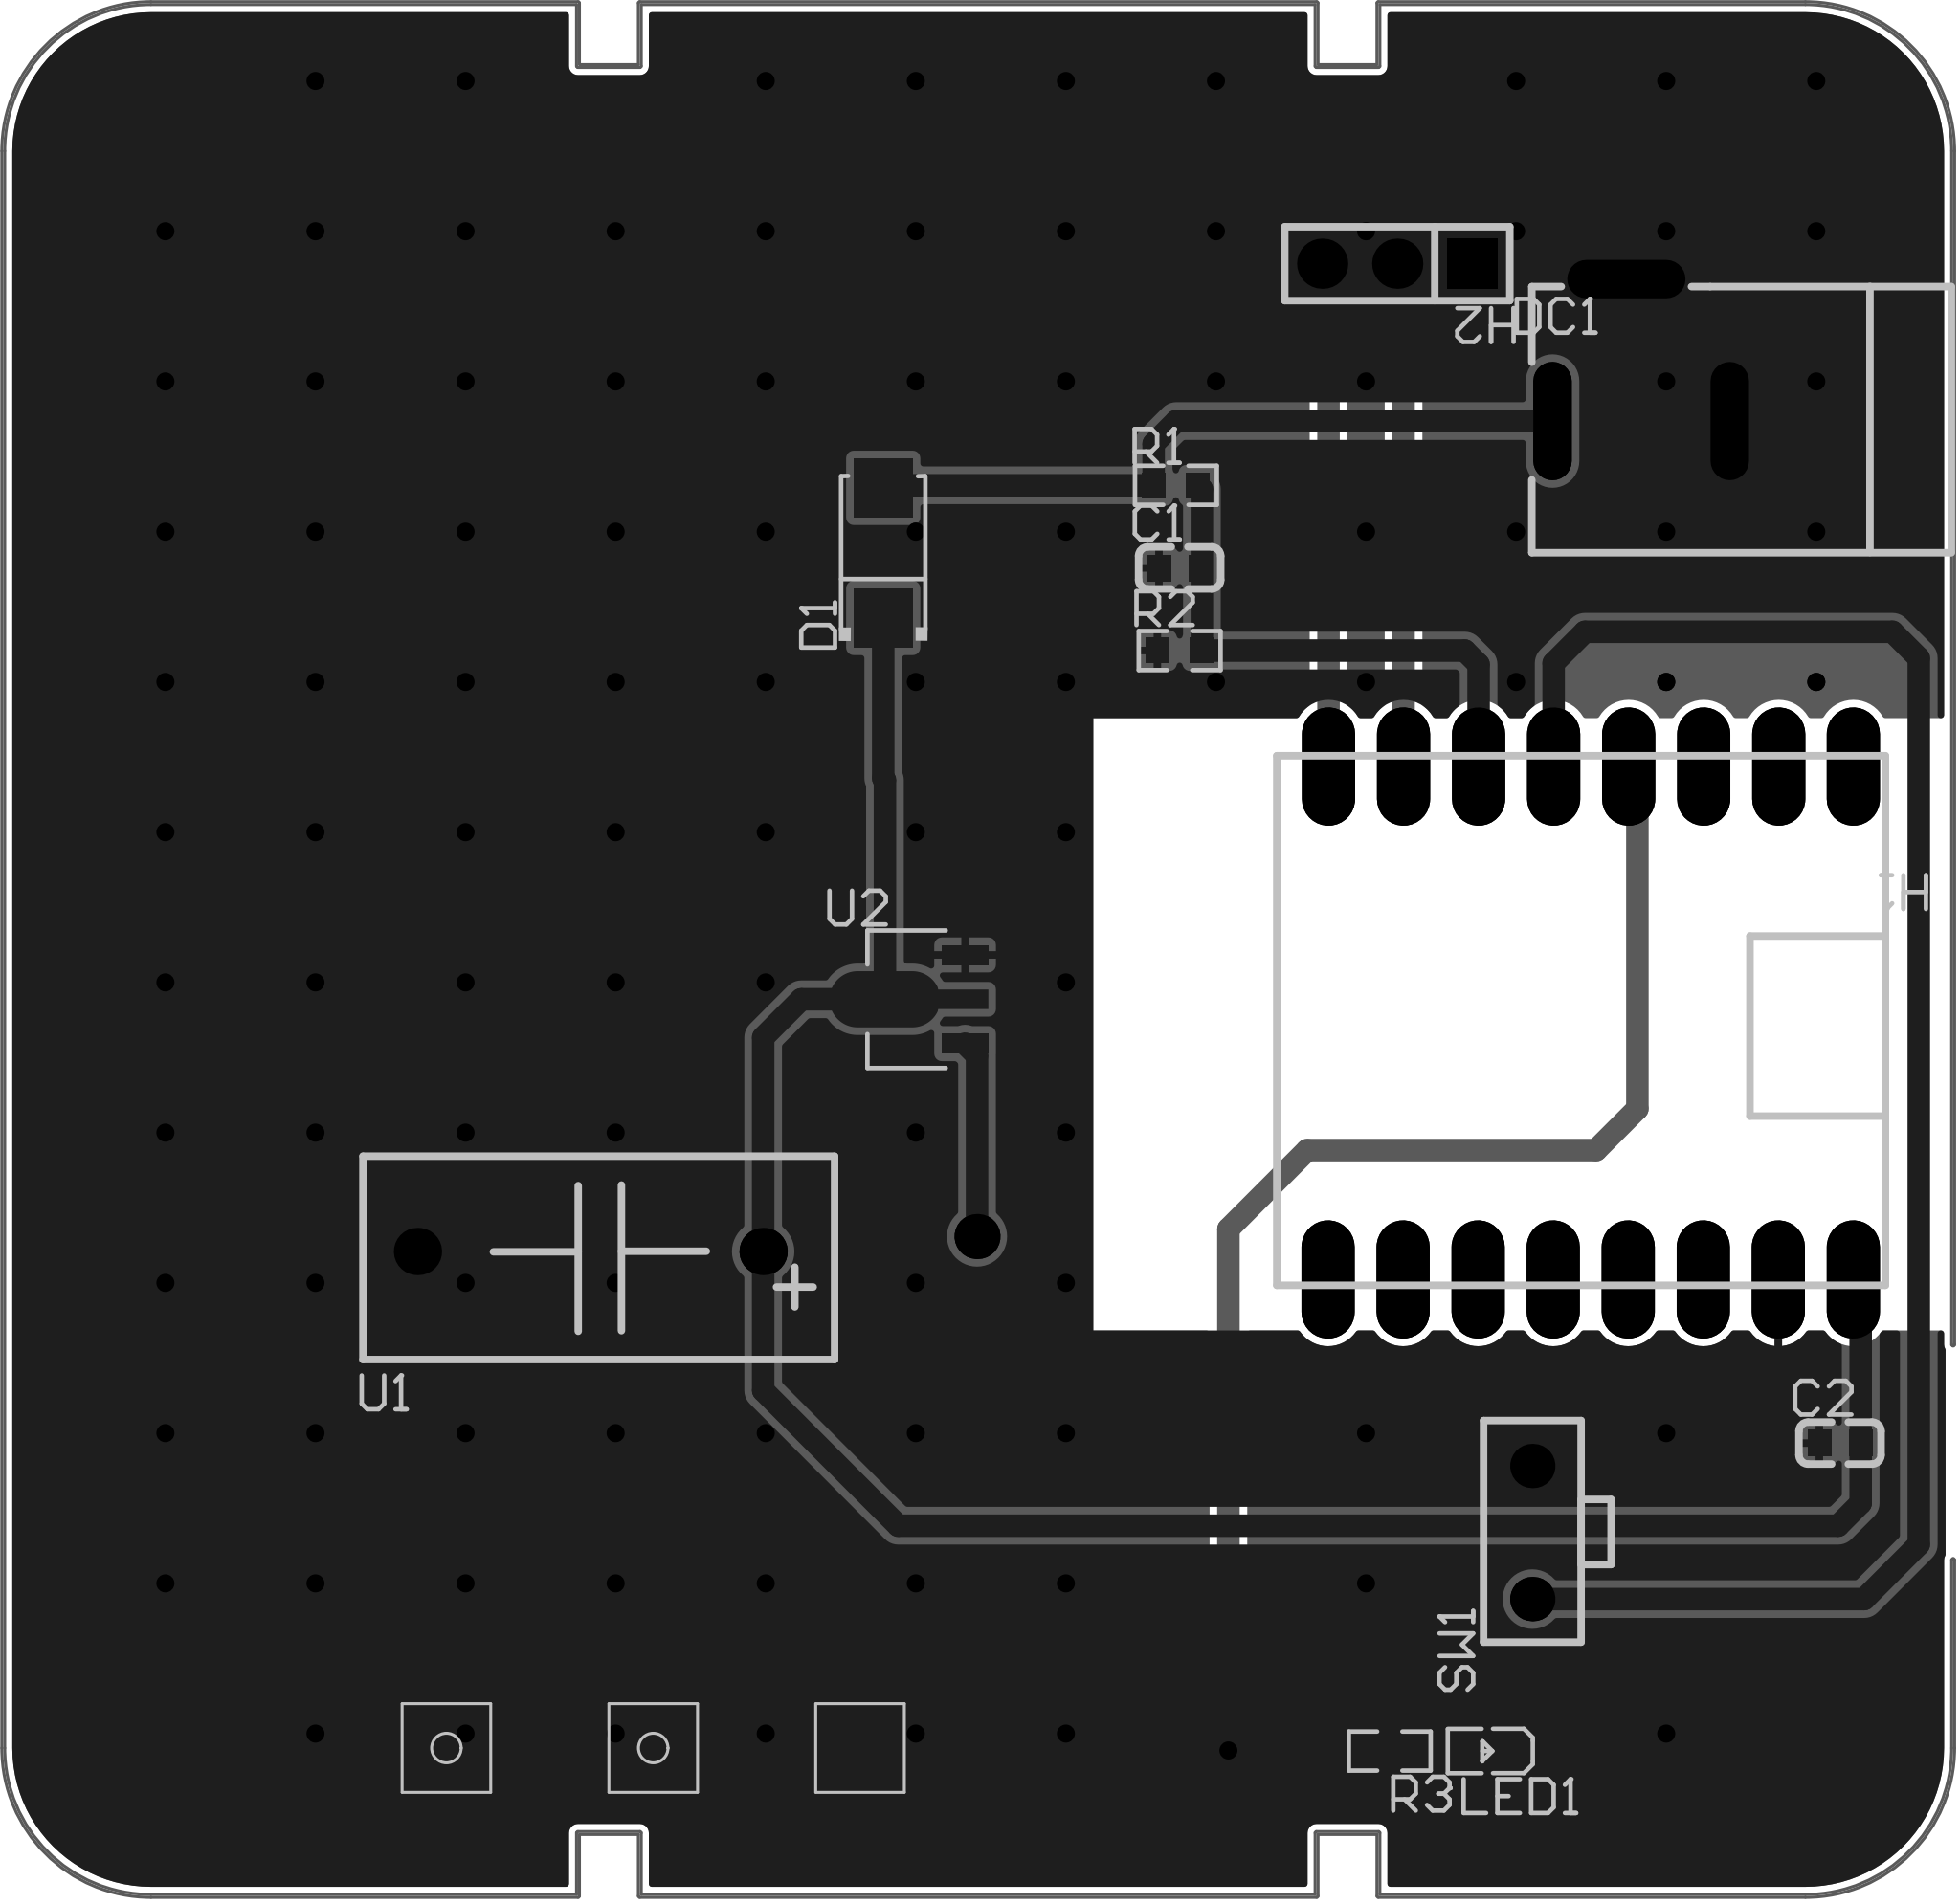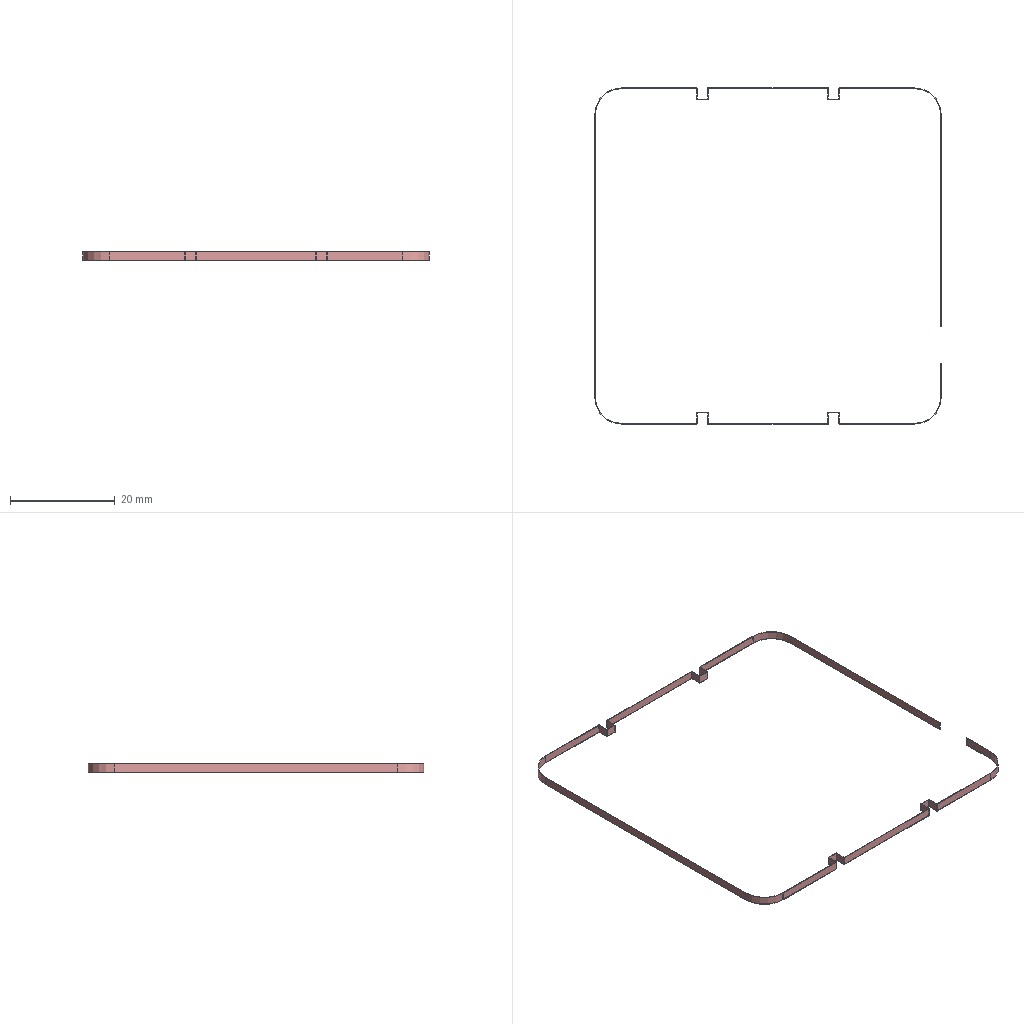Circuit board layout | Altium Designer | box 66.1 x 64.1 x 1.6 mm
Layer stack:
# Altium Designer layer stack of  (unit mm; dielectric type: 0 none, 1 core, 2 prepreg, 3 surface material)
index,name,kind,layer,copper_thickness_mm,dielectric_type,dielectric_thickness_mm,dielectric_material,dielectric_constant
0,Top Paste Mask Layer,other,,,,,,
1,Top Silkscreen Layer,other,,,,,,
2,Top Solder Mask Layer,dielectric,,,3,0.01,,3.3
3,Top Layer,copper,Top Layer,0.035,,,,
4,Dielectric1,dielectric,,,3,1.51,FR4,4.5
5,Bottom Layer,copper,Bottom Layer,0.035,,,,
6,Bottom Solder Mask Layer,dielectric,,,3,0.01,,3.3
7,Bottom Silkscreen Layer,other,,,,,,
8,Bottom Paste Mask Layer,other,,,,,,
# drill layer pairs: low layer,high layer
drill_pair,Top Layer,Bottom Layer
Part placement:
Designator,Comment,Layer,Footprint,Center-X(mm),Center-Y(mm),Rotation
C1,100nF,TopLayer,C0603,125.984,131.191,0
C2,100nF,TopLayer,C0603,148.336,101.6,0
D1,SS34,TopLayer,SMA_L4.3-W2.6-LS5.2-RD,115.951,131.699,90
H1,,TopLayer,HDR-TH_16P-P2.54-V-F-R2-C8-S2.54-1,139.898,115.803,180
R1,10K,TopLayer,R0603,125.857,133.985,180
R2,15K,TopLayer,R0603,125.984,128.397,0
R3,1K,TopLayer,R0603,133.096,91.186,0
U1,2F,TopLayer,CAP-TH_BD8.0-P3.50-D0.6-FD_GDC02R7R205LD0816,106.037,108.077,180
U2,HT7033A-1,TopLayer,SOT-89-3_L4.5-W2.5-P1.50-LS4.2-BR,117.561,116.606,0
DC1,,TopLayer,DC-2.0,141.605,138.557,0
H2,,TopLayer,HDR-TH_3P-P2.54-V-M,133.35,141.478,180
LED1,,TopLayer,LED_0603,136.449,91.194,180
SW1,,TopLayer,Key_TH_3.5x6x4.3,137.922,98.574,90
Pad and via stacks:
# Altium Designer via and pad stacks of  (unit mm). Each distinct definition once, with the count of objects using it.
# via: kind,start_layer,end_layer,hole_mm,diameter_mm,mode(0 simple;1 top-mid-bottom;2 full stack),diameter_per_layer,count,example_net
# pad: kind,layer,hole_mm,hole_type(0 round;1 square;2 slot),plating,top_size,top_shape(1 round;2 rect;3 octagon;9 rounded rect),mid_size,bottom_size,mode,footprint,size_per_layer,count,example
pad,Top Layer,0,0,plated,0.8x0.9,2,0.8x0.9,0.8x0.9,0,C0603,,4,C1.2
pad,Top Layer,0,0,plated,2x2,2,2x2,2x2,0,SMA_L4.3-W2.6-LS5.2-RD,,2,D1.2
pad,Top Layer,0,0,plated,0.8065x0.864,2,0.8065x0.864,0.8065x0.864,0,R0603,,6,R1.2
pad,Top Layer,0,0,plated,1.575x0.672,2,1.575x0.672,1.575x0.672,0,SOT-89-3_L4.5-W2.5-P1.50-LS4.2-BR,,2,U2.1
pad,Top Layer,0,0,plated,0.95x0.95,1,0.95x0.95,0.95x0.95,0,SOT-89-3_L4.5-W2.5-P1.50-LS4.2-BR,,1,U2.2
pad,Top Layer,0,0,plated,0.8001x0.8001,2,0.8001x0.8001,0.8001x0.8001,0,LED_0603,,2,LED1.1
pad,Multi-Layer,1.1,0,plated,1.8x4,1,1.8x4,1.8x4,0,HDR-TH_16P-P2.54-V-F-R2-C8-S2.54-1,,16,H1.15
pad,Multi-Layer,1,0,plated,1.6x1.6,1,1.6x1.6,1.6x1.6,0,CAP-TH_BD8.0-P3.50-D0.6-FD_GDC02R7R205LD0816,,2,U1.1
pad,Multi-Layer,0.9144,0,plated,1.524x1.524,1,1.524x1.524,1.524x1.524,0,,,1,1
pad,Multi-Layer,0.8001,2,plated,4x1.3,1,4x1.3,4x1.3,0,DC-2.0,,3,DC1.2
pad,Multi-Layer,1.1,0,plated,1.7x1.7,2,1.7x1.7,1.7x1.7,0,HDR-TH_3P-P2.54-V-M,,1,H2.1
pad,Multi-Layer,1.1,0,plated,1.7x1.7,1,1.7x1.7,1.7x1.7,0,HDR-TH_3P-P2.54-V-M,,2,H2.2
pad,Multi-Layer,1,0,plated,1.5x1.5,1,1.5x1.5,1.5x1.5,0,Key_TH_3.5x6x4.3,,2,SW1.A
via,Top Layer,Bottom Layer,0.3048,0.61,0,,105,$1N5
Copper pours:
name,layer,net,type(0 solid;1 hatched;2 none)
Top Layer-GND,Top Layer,GND,0
Bottom Layer-GND,Bottom Layer,GND,0
Design rules, without the lines most boards share:
# Altium Designer design rules of  (exported by Altium Designer, unit mm)
# columns: name | kind | enabled | priority | scope1 | scope2 | descriptor | typed fields (field=value)
creepage | 65 | enabled | 1 | All | All | Creepage Distance Constraint =(0mil) (All),(All) |
copperRegion | 20 | enabled | 1 | (InNet('GND')) | All | Polygon Connect Rule(Relief Connect )(Conductor Width=10mil) (Relief Angle=90 Angle) (Entries=4) (Air Gap Width=10mil) ((InNet('GND'))),(All) | connect_style(0=relief,1=direct,2=none)=0 relief_conductor_width=0.254 relief_entries=4